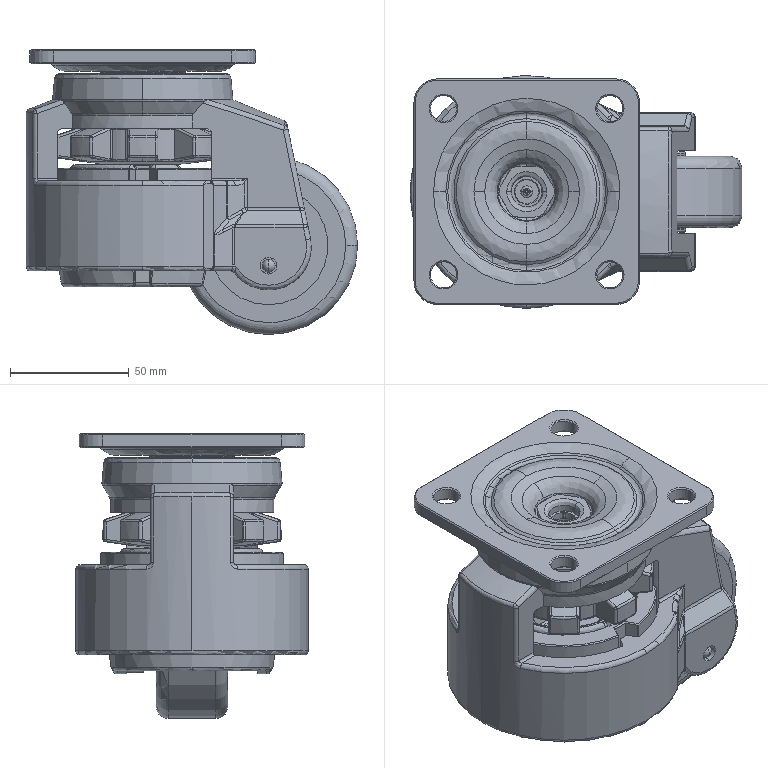Part | SolidWorks | features BaseBody 7 | 7 solids | 1480 faces | box 139.5 x 98 x 120 mm | volume 590754 mm3 | spline 494 | cylinder 362 | plane 346 | cone 199 | torus 73 | sphere 6 | commonest cylinder face diameters 2 x88 4 x67 1 x26 5.5 x12 75 x11 14 x10